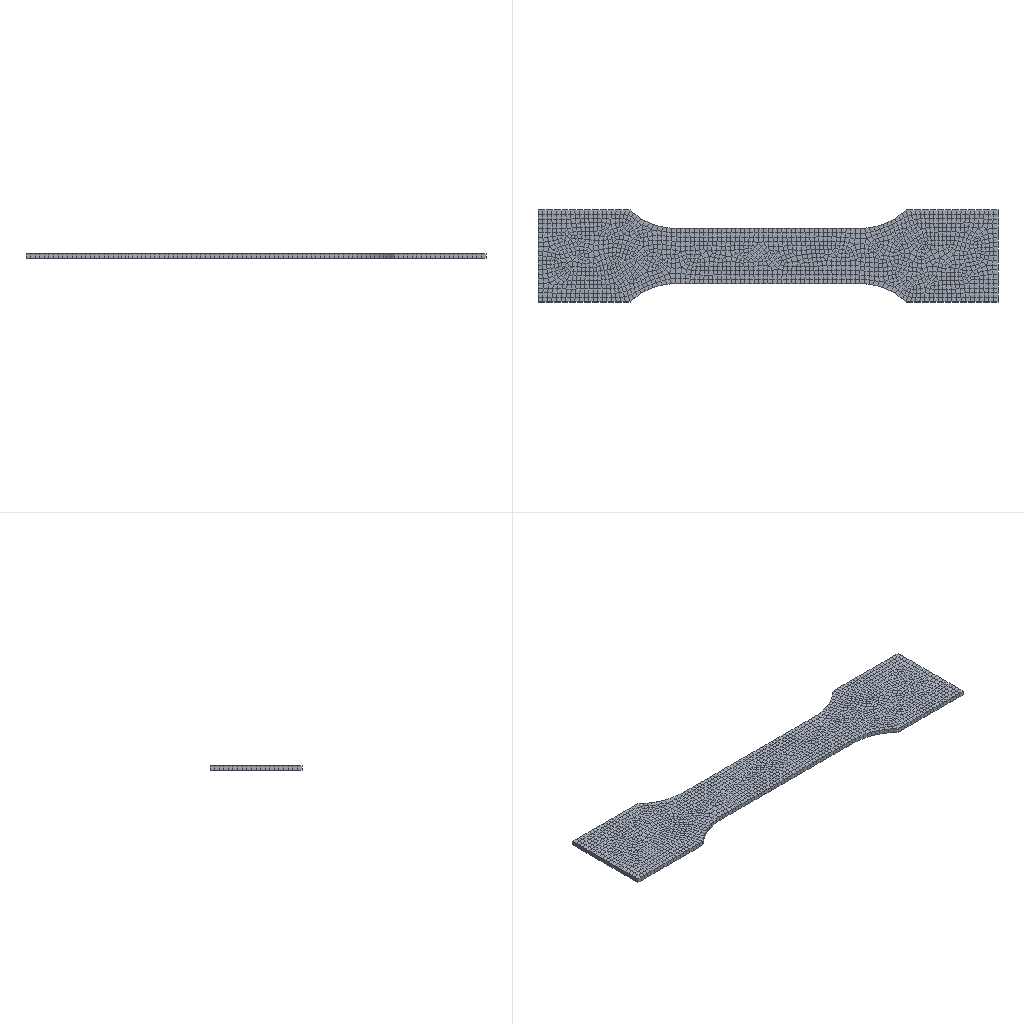Simulation study | abaqus
Set-up summary:
category,name,step,type,value,unit,region
solver,abaqus
solver,version,,,Abaqus/Standard 2020
units,not stated in the deck,,not stated
analysis,deck,,static,static
load_step,Step-1,Step-1,static,nlgeom=False
contact,interactions,,,general=0 pairs=0 ties=0
load_step,requested,,,1
mesh,nodes,,,3950
mesh,elements,,,1852
element_type,C3D8R,,solid,1852
load,load commands in deck,,count,1
bc,support commands in deck,,count,1
material,MATERIAL-1,,in results
check,setup vs results,,match,"per instance, exact: element labels, types and connectivity; labels of the nodes the elements use; coordinates of those nodes at SINGLE_PRECISION in 1 of 1 instance(s)"
Abaqus input file, long lists of numbers shortened:
*Heading
** Job name: Job-1 Model name: Model-1
** Generated by: Abaqus/CAE 2020
*Preprint, echo=NO, model=NO, history=NO, contact=NO
**
** PARTS
**
*Part, name=Part-1
*Node
      1,          -1.,           3.,           0.
      2,         -2.5,           3.,           0.
** (3948 more lines like these left out)
*Element, type=C3D8R
   1,  714,  565,  506,   61, 2689, 2540, 2481, 2036
   2,  992,  343,  856,  903, 2967, 2318, 2831, 2878
** (1850 more lines like these left out)
*Nset, nset=Set-1, generate
    1,  3950,     1
*Elset, elset=Set-1, generate
    1,  1852,     1
** Section: Section-1
*Solid Section, elset=Set-1, material=Material-1
,
*End Part
**
*Part, name=crack
*End Part
**
**
** ASSEMBLY
**
*Assembly, name=Assembly
**
*Instance, name=Part-1-1, part=Part-1
*End Instance
**
*Instance, name=crack-1, part=crack
          0.,          -1.,          0.5
          0.,          -1.,          0.5,           0., 1.26880521644779e-08,          0.5, 90.
*End Instance
**
*Nset, nset=Set-1, instance=Part-1-1
   77,   78,   79,   80,   81,   82,   83,   84,   85,  531,  532,  533,  534,  535,  536,  537
  538,  539,  540,  541,  542, 2052, 2053, 2054, 2055, 2056, 2057, 2058, 2059, 2060, 2506, 2507
** (1 more lines like these left out)
*Elset, elset=Set-1, instance=Part-1-1
  65, 329, 330, 354, 360, 365, 367, 768, 770, 771, 772, 773, 774, 775, 776, 855
 860, 862, 880, 928
*Nset, nset=_PickedSet8, internal, instance=Part-1-1, generate
    1,  3950,     1
*Elset, elset=_PickedSet8, internal, instance=Part-1-1, generate
    1,  1852,     1
*Elset, elset=_Surf-1_S6, internal, instance=Part-1-1
 181,
*Elset, elset=_Surf-1_S5, internal, instance=Part-1-1
 185, 498, 726, 829, 830, 832, 833, 834, 872, 902
*Elset, elset=_Surf-1_S3, internal, instance=Part-1-1
 490, 723, 724, 725, 727, 729, 730, 831
*Elset, elset=_Surf-1_S4, internal, instance=Part-1-1
 722,
*Surface, type=ELEMENT, name=Surf-1
_Surf-1_S6, S6
_Surf-1_S5, S5
_Surf-1_S4, S4
_Surf-1_S3, S3
*Enrichment, name=Crack-1, type=STATIONARY CRACK, elset=_PickedSet8
*End Assembly
*Amplitude, name=Amp-1
             0.,              0.,              1.,              1.
**
** MATERIALS
**
*Material, name=Material-1
*Damage Initiation, criterion=MAXPS
30.,
*Damage Evolution, type=DISPLACEMENT
 1e-09,
*Density
 2.5e-09,
*Elastic
65000., 0.27
*Initial Conditions, type=ENRICHMENT
Part-1-1.165, 1,Crack-1, -0.5214, 0.1228
Part-1-1.165, 2,Crack-1, -0.2987, -0.192
Part-1-1.165, 3,Crack-1, 0.01565, -0.004065
Part-1-1.165, 4,Crack-1, -0.191, 0.3562
Part-1-1.165, 5,Crack-1, -0.5214, 0.1228
Part-1-1.165, 6,Crack-1, -0.2987, -0.192
Part-1-1.165, 7,Crack-1, 0.01565, -0.004065
Part-1-1.165, 8,Crack-1, -0.191, 0.3562
Part-1-1.133, 1,Crack-1, 0.01565
Part-1-1.133, 2,Crack-1, -0.2987
Part-1-1.133, 3,Crack-1, -0.1519
Part-1-1.133, 4,Crack-1, 0.2128
Part-1-1.133, 5,Crack-1, 0.01565
Part-1-1.133, 6,Crack-1, -0.2987
Part-1-1.133, 7,Crack-1, -0.1519
Part-1-1.133, 8,Crack-1, 0.2128
Part-1-1.181, 1,Crack-1, 0.2128
Part-1-1.181, 2,Crack-1, -0.1519
Part-1-1.181, 3,Crack-1, 0.01351
Part-1-1.181, 4,Crack-1, 0.4268
Part-1-1.181, 5,Crack-1, 0.2128
Part-1-1.181, 6,Crack-1, -0.1519
Part-1-1.181, 7,Crack-1, 0.01351
Part-1-1.181, 8,Crack-1, 0.4268
Part-1-1.254, 1,Crack-1, -0.1519
Part-1-1.254, 2,Crack-1, -0.5733
Part-1-1.254, 3,Crack-1, -0.5381
Part-1-1.254, 4,Crack-1, 0.01351
Part-1-1.254, 5,Crack-1, -0.1519
Part-1-1.254, 6,Crack-1, -0.5733
Part-1-1.254, 7,Crack-1, -0.5381
Part-1-1.254, 8,Crack-1, 0.01351
Part-1-1.253, 1,Crack-1, 0.01351
Part-1-1.253, 2,Crack-1, -0.5381
Part-1-1.253, 3,Crack-1, -0.5298
Part-1-1.253, 4,Crack-1, -0.03328
Part-1-1.253, 5,Crack-1, 0.01351
Part-1-1.253, 6,Crack-1, -0.5381
Part-1-1.253, 7,Crack-1, -0.5298
Part-1-1.253, 8,Crack-1, -0.03328
** (40 more lines like these left out)
** ----------------------------------------------------------------
**
** STEP: Step-1
**
*Step, name=Step-1, nlgeom=NO, inc=1000
*Static
0.01, 1., 1e-05, 0.1
**
** BOUNDARY CONDITIONS
**
** Name: BC-1 Type: 对称/反对称/完全固定
*Boundary
Set-1, ENCASTRE
**
** LOADS
**
** Name: Load-1   Type: Pressure
*Dsload, amplitude=Amp-1
Surf-1, P, -50.
**
** OUTPUT REQUESTS
**
*Restart, write, frequency=0
**
** FIELD OUTPUT: F-Output-1
**
*Output, field
*Node Output
CF, PHILSM, PSILSM, RF, U, V
*Element Output, directions=YES
E, EACTIVE, ENRRTXFEM, LE, LOADSXFEM, MISES, MISESMAX, MISESONLY, PE, PEEQ, PEMAG, PRESSONLY, S, SDEG, SEQUT, SSAVG
STATUS, STATUSXFEM, YIELDPOT
*Contact Output
CDISP, CSTRESS
*Output, history, frequency=0
**
** HISTORY OUTPUT: H-Output-1
**
*Contour Integral, crack name=Crack-1, contours=5, type=K FACTORS, xfem
*End Step
Results summary:
result,step,,completed,increments=15 time=1.0/1.0
result,analysis,,,static
result,last_loadstep,,,1
result,analysis steps,,count,1
result,primary field,,,U
result,reaction total,,FX,-250,model units
result,reaction total,,FY,0.0,model units
result,reaction total,,FZ,0.0,model units